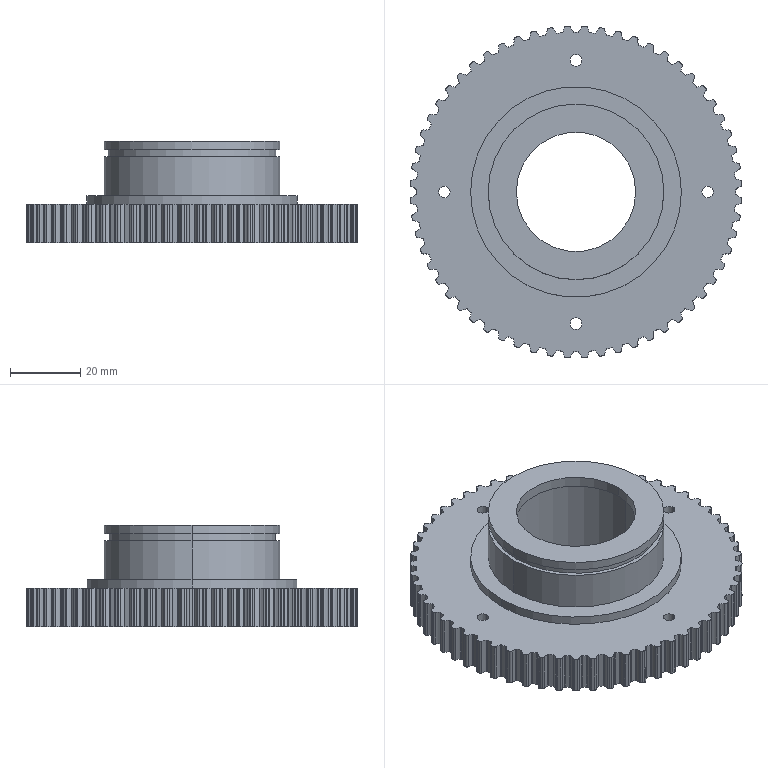Part | STEP file | EBJ01-S5M100-60-A-H-d14 twist driven pulley SGN-4-05 (threaded type) | 1 solid | 560 faces | box 94.44 x 94.44 x 29 mm | volume 75497 mm3 | cylinder 553 | plane 7 | commonest cylinder face diameters 1.1 x146 0.5 x138 6.55 x128 90.99 x61 94.53 x60 3.3 x8